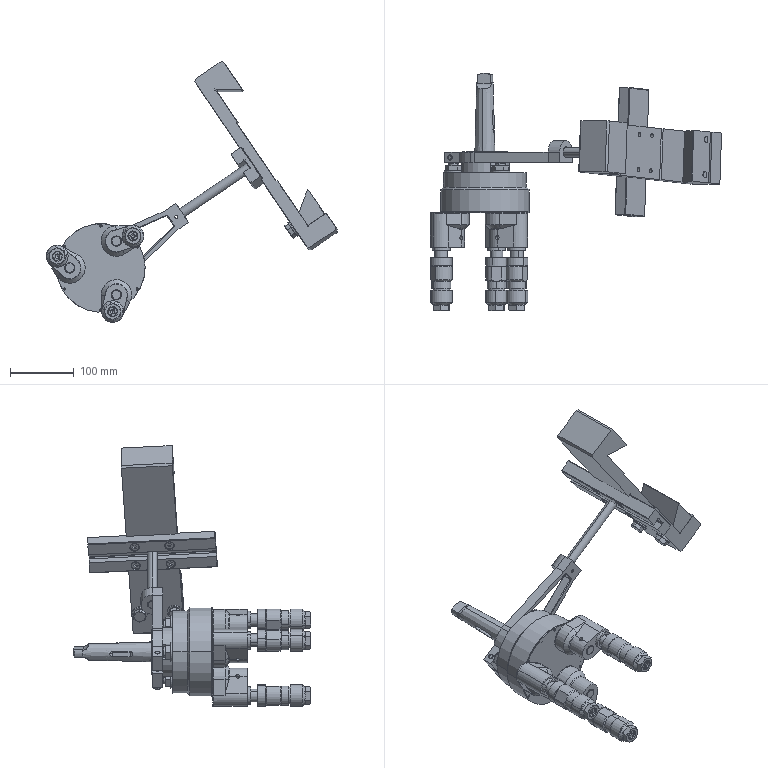Part | SolidWorks | features ReferencePattern 32, CompositeCurve 27, LocalCirPattern 3 | 70 solids | 2781 faces | box 456.998 x 372.31 x 409.469 mm | volume 2395331 mm3 | cylinder 1384 | plane 590 | cone 443 | torus 226 | sphere 136 | spline 2 | commonest cylinder face diameters 8.722 x114 8.208 x108 23.086 x96 21.75 x54 28.5 x54 18 x48